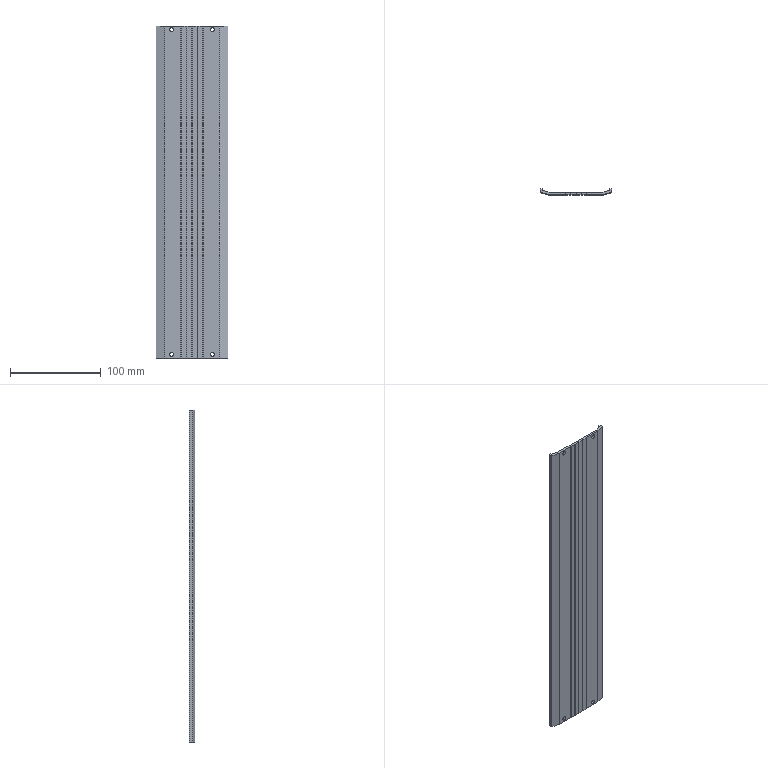Part | STEP file | 1.5Z axis cover plate_3X cover plate | 1 solid | 37 faces | box 79 x 6 x 366 mm | volume 77305 mm3 | plane 29 | cylinder 8 | commonest cylinder face diameters 4.2 x8